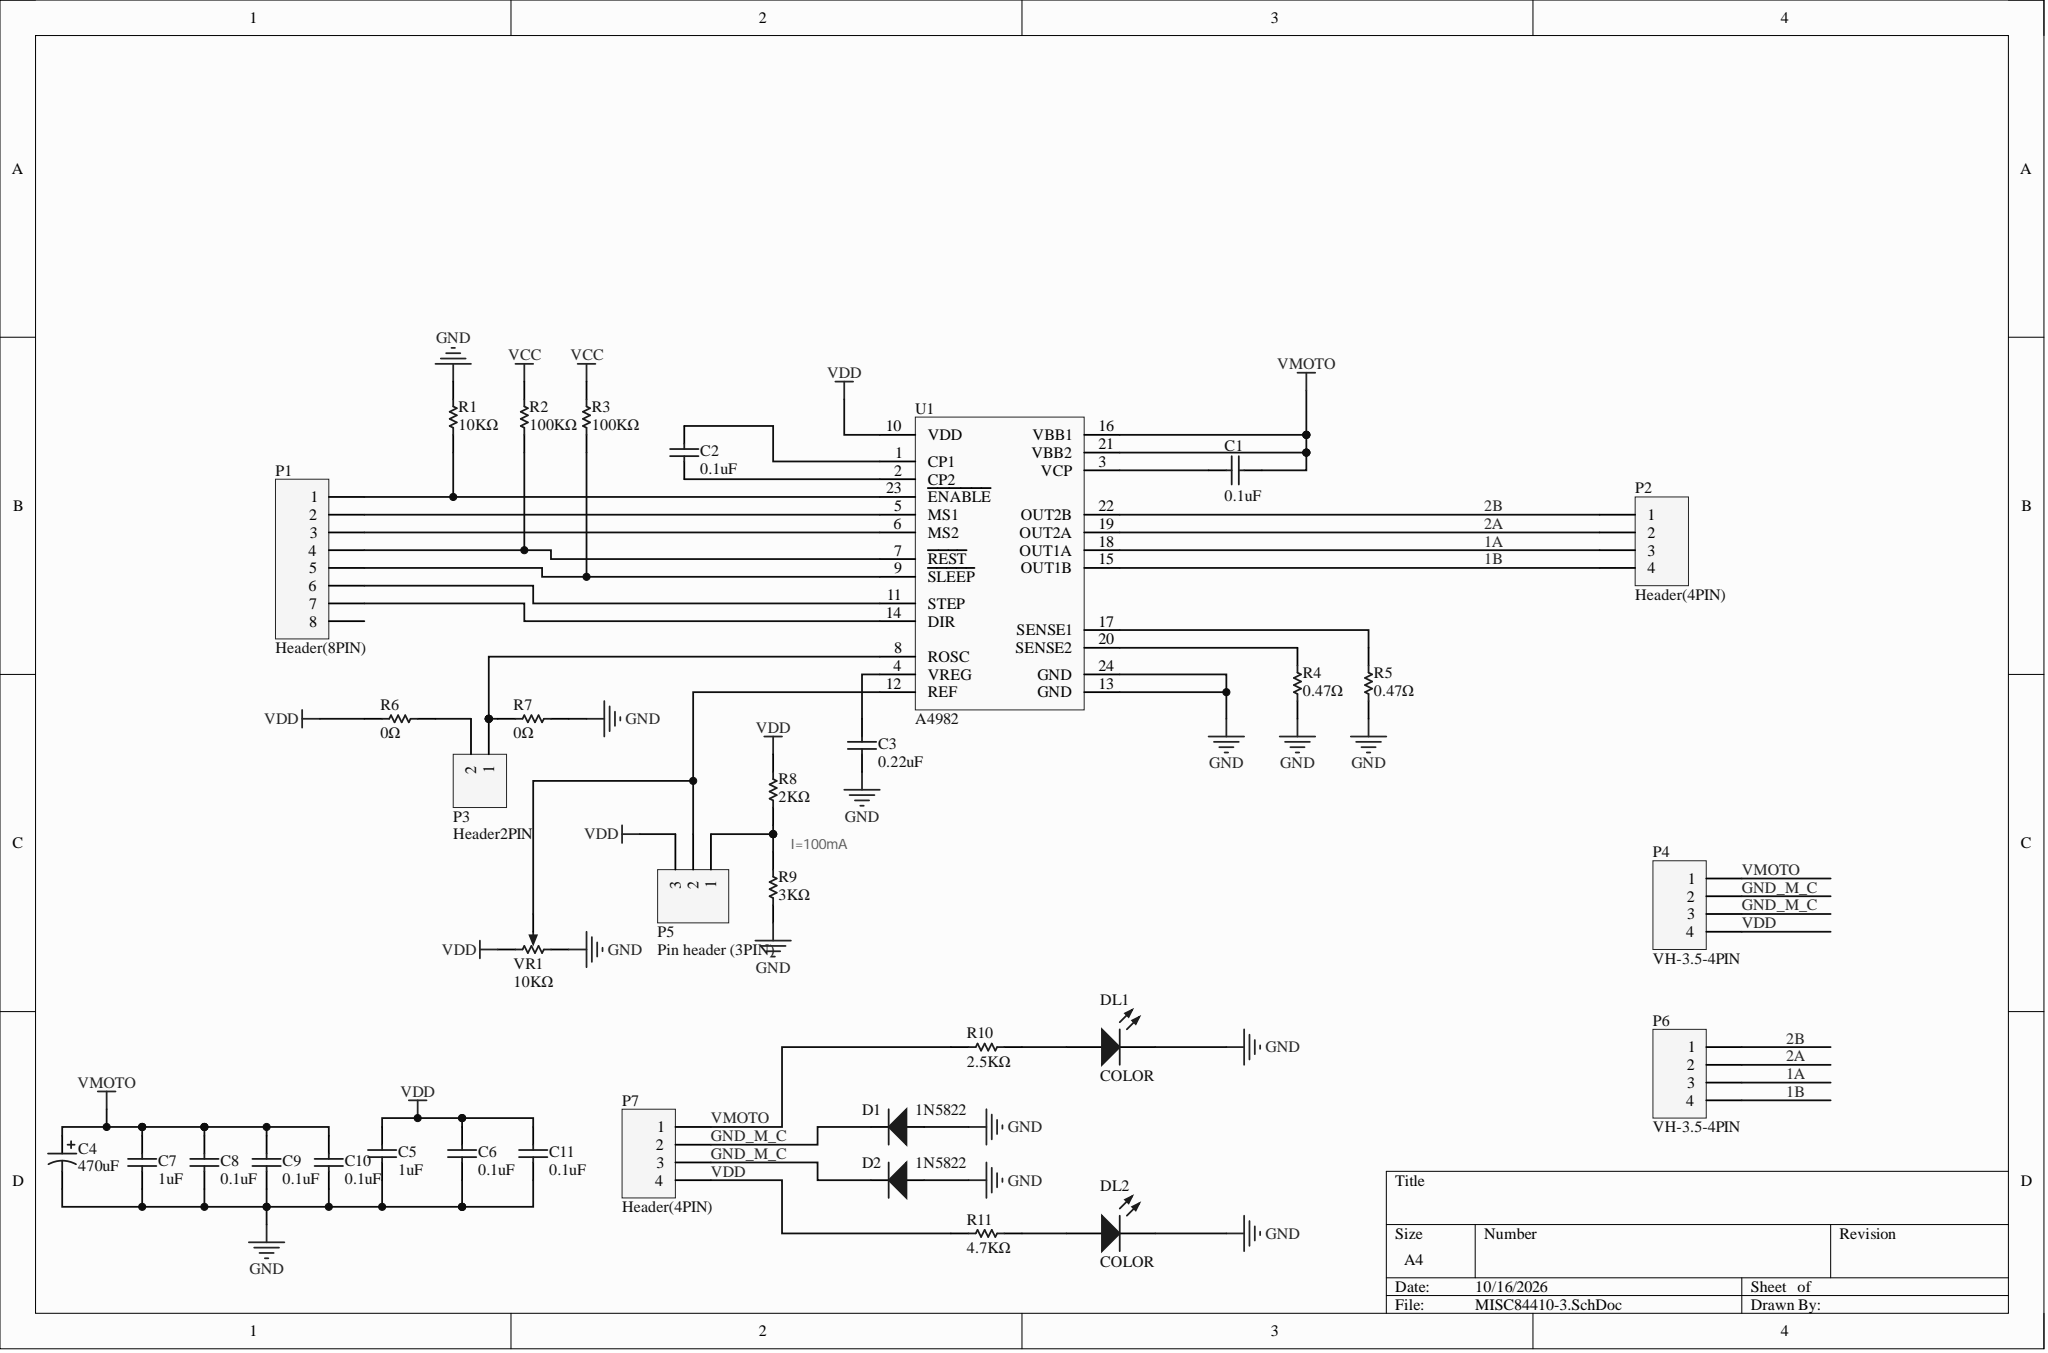Circuit board | Altium Designer | 35 parts | 28 nets
Bill of materials:
Comment,Description,Designator,Footprint,LibRef,Quantity
"0.1uF","0805 SMD capacitor","C1, C2, C6, C8, C9, C10, C11","0805C","CAP0805","7"
"0.22uF","0805 SMD capacitor","C3","0805C","CAP0805","1"
"470uF","THT capacitor","C4","CAP-SMD Aluminum Capacitors F8 220uF 35V","CAP-AEC","1"
"1uF","0805 SMD capacitor","C5, C7","0805C","CAP0805","2"
"1N5822","1N5822","D1, D2","1N5822","IN5822","2"
"COLOR","LED_0805","DL1, DL2","0805D","LED_0805","2"
"Header(8PIN)","Header, 8-Pin","P1","排针（8PIN）","Header 8","1"
"Header(4PIN)","Header, 4-Pin","P2, P7","排针(4PIN)","Header 4","2"
"Header2PIN","Header, 2-Pin","P3","排针2PIN","Header 2","1"
"VH-3.5-4PIN","Header, 4-Pin","P4, P6","VH-3.5-4PIN","Header 4","2"
"Pin header (3PIN)","Pin header (3PIN)","P5","排针(3PIN)","Header 3","1"
"10KΩ","0805 SMD resistor","R1","0805R","RES0805","1"
"100KΩ","0805 SMD resistor","R2, R3","0805R","RES0805","2"
"0.47Ω","0805 SMD resistor","R4, R5","0805R","RES0805","2"
"0Ω","0805 SMD resistor","R6, R7","0805R","RES0805","2"
"2KΩ","0805 SMD resistor","R8","0805R","RES0805","1"
"3KΩ","0805 SMD resistor","R9","0805R","RES0805","1"
"2.5KΩ","0805 SMD resistor","R10","0805R","RES0805","1"
"4.7KΩ","0805 SMD resistor","R11","0805R","RES0805","1"
"Value","A4982","U1","A4982","A4982","1"
"10KΩ","RPOT-SMD-10KΩ","VR1","3224W","RPOT","1"
Netlist (Protel format):
[
C1
0805C
0.1uF



]
[
C2
0805C
0.1uF



]
[
C3
0805C
0.22uF



]
[
C4
CAP-SMD Aluminum Capacitors F8 220uF 35V
470uF



]
[
C5
0805C
1uF



]
[
C6
0805C
0.1uF



]
[
C7
0805C
1uF



]
[
C8
0805C
0.1uF



]
[
C9
0805C
0.1uF



]
[
C10
0805C
0.1uF



]
[
C11
0805C
0.1uF



]
[
D1
1N5822
1N5822



]
[
D2
1N5822
1N5822



]
[
DL1
0805D
COLOR



]
[
DL2
0805D
COLOR



]
[
P1
排针（8PIN）
Header(8PIN)



]
[
P2
排针(4PIN)
Header(4PIN)



]
[
P3
排针2PIN
Header2PIN



]
[
P4
VH-3.5-4PIN
VH-3.5-4PIN



]
[
P5
排针(3PIN)
Pin header (3PIN)



]
[
P6
VH-3.5-4PIN
VH-3.5-4PIN



]
[
P7
排针(4PIN)
Header(4PIN)



]
[
R1
0805R
10KΩ



]
[
R2
0805R
100KΩ



]
[
R3
0805R
100KΩ



]
[
R4
0805R
0.47Ω



]
[
R5
0805R
0.47Ω



]
[
R6
0805R
0Ω



]
[
R7
0805R
0Ω



]
[
R8
0805R
2KΩ



]
[
R9
0805R
3KΩ



]
[
R10
0805R
2.5KΩ



]
[
R11
0805R
4.7KΩ



]
[
U1
A4982
Value



]
[
VR1
3224W
10KΩ



]
(
VMOTO
C1-1
C4-1
C7-1
C8-1
C9-1
C10-1
P4-1
P7-1
R10-1
U1-16
U1-21
)
(
VDD
C5-1
C6-1
C11-1
P4-4
P5-3
P7-4
R6-2
R8-1
R11-1
U1-10
VR1-3
)
(
VCC
R2-2
R3-2
)
(
NetR5_2
R5-2
U1-17
)
(
NetR4_2
R4-2
U1-20
)
(
NetP5_2
P5-2
U1-12
VR1-2
)
(
NetP5_1
P5-1
R8-2
R9-1
)
(
NetP3_2
P3-2
R6-1
)
(
NetP3_1
P3-1
R7-2
U1-8
)
(
NetP1_7
P1-7
U1-14
)
(
NetP1_6
P1-6
U1-11
)
(
NetP1_5
P1-5
R3-1
U1-9
)
(
NetP1_4
P1-4
R2-1
U1-7
)
(
NetP1_3
P1-3
U1-6
)
(
NetP1_2
P1-2
U1-5
)
(
NetP1_1
P1-1
R1-1
U1-23
)
(
NetDL2_1
DL2-1
R11-2
)
(
NetDL1_1
DL1-1
R10-2
)
(
NetC3_1
C3-1
U1-4
)
(
NetC2_2
C2-2
U1-1
)
(
NetC2_1
C2-1
U1-2
)
(
NetC1_2
C1-2
U1-3
)
(
GND_M_C
D1-2
D2-2
P4-2
P4-3
P7-2
P7-3
)
(
GND
C3-2
C4-2
C5-2
C6-2
C7-2
C8-2
C9-2
C10-2
C11-2
D1-1
D2-1
DL1-2
DL2-2
R1-2
R4-1
R5-1
R7-1
R9-2
U1-13
U1-24
VR1-1
)
(
2B
P2-1
P6-1
U1-22
)
(
2A
P2-2
P6-2
U1-19
)
(
1B
P2-4
P6-4
U1-15
)
(
1A
P2-3
P6-3
U1-18
)